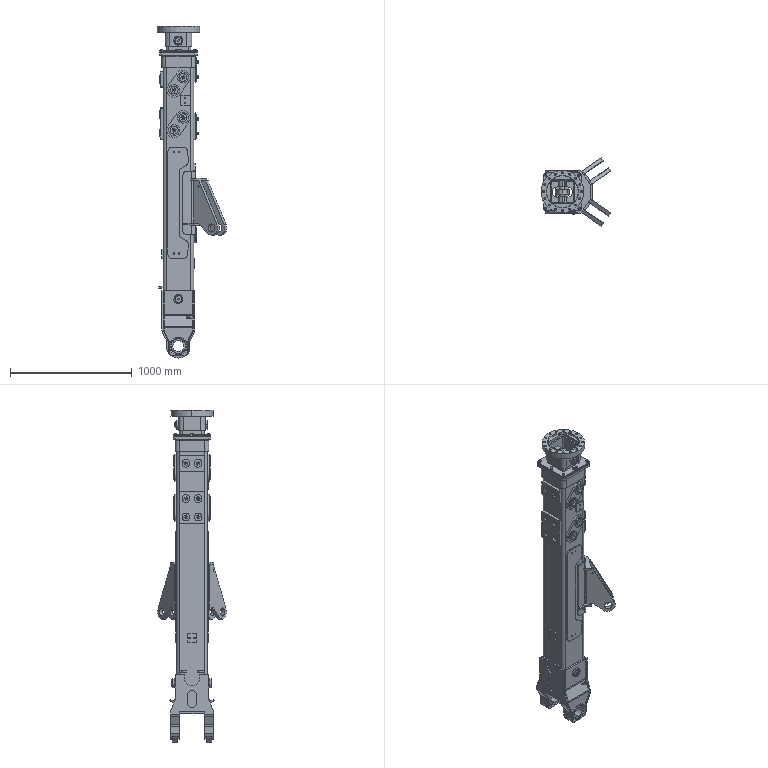Part | SolidWorks | 172 solids | 4527 faces | volume 96493183 mm3 | plane 2042 | cylinder 1435 | cone 818 | torus 224 | spline 8 | commonest cylinder face diameters 10 x132 60 x100 64 x100 10.2 x96 80 x79 2 x72